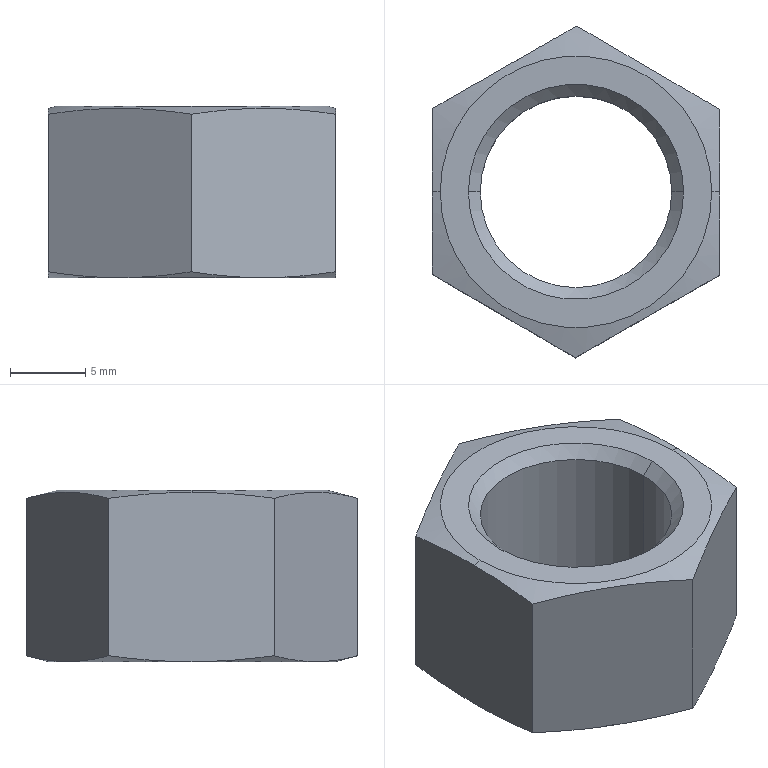Part | SolidWorks | features Cut 2, Chamfer 1, Extrusion 1 | 1 solid | 18 faces | box 19.096 x 22 x 11.38 mm | volume 2097 mm3 | cone 8 | plane 8 | cylinder 2 | commonest cylinder face diameters 12.7 x2
STEP:
#1=CARTESIAN_POINT('',(-6.35,0.,10.594));
#2=VERTEX_POINT('',#1);
#3=CARTESIAN_POINT('',(6.35,0.,10.594));
#4=VERTEX_POINT('',#3);
#5=CARTESIAN_POINT('',(0.,0.,10.594));
#6=DIRECTION('',(0.,0.,1.));
#7=DIRECTION('',(-1.,0.,0.));
#8=AXIS2_PLACEMENT_3D('',#5,#6,#7);
#9=CIRCLE('',#8,6.35);
#10=EDGE_CURVE('',#2,#4,#9,.T.);
#11=ORIENTED_EDGE('',*,*,#10,.F.);
#12=CARTESIAN_POINT('',(-7.136,0.,11.38));
#13=VERTEX_POINT('',#12);
#14=CARTESIAN_POINT('',(-6.35,0.,10.594));
#15=DIRECTION('',(-0.7071,0.,0.7071));
#16=VECTOR('',#15,1000.);
#17=LINE('',#14,#16);
#18=EDGE_CURVE('',#2,#13,#17,.T.);
#19=ORIENTED_EDGE('',*,*,#18,.T.);
#20=CARTESIAN_POINT('',(7.136,0.,11.38));
#21=VERTEX_POINT('',#20);
#22=CARTESIAN_POINT('',(0.,0.,11.38));
#23=DIRECTION('',(0.,0.,-1.));
#24=DIRECTION('',(-1.,0.,0.));
#25=AXIS2_PLACEMENT_3D('',#22,#23,#24);
#26=CIRCLE('',#25,7.136);
#27=EDGE_CURVE('',#21,#13,#26,.T.);
#28=ORIENTED_EDGE('',*,*,#27,.F.);
#29=CARTESIAN_POINT('',(6.35,0.,10.594));
#30=DIRECTION('',(0.7071,0.,0.7071));
#31=VECTOR('',#30,1000.);
#32=LINE('',#29,#31);
#33=EDGE_CURVE('',#4,#21,#32,.T.);
#34=ORIENTED_EDGE('',*,*,#33,.F.);
#35=EDGE_LOOP('',(#11,#19,#28,#34));
#36=FACE_OUTER_BOUND('',#35,.T.);
#37=CARTESIAN_POINT('',(0.,0.,10.594));
#38=DIRECTION('',(0.,0.,1.));
#39=DIRECTION('',(1.,0.,0.));
#40=AXIS2_PLACEMENT_3D('',#37,#38,#39);
#41=CONICAL_SURFACE('',#40,6.35,0.7854);
#42=ADVANCED_FACE('',(#36),#41,.F.);
#43=CARTESIAN_POINT('',(6.35,0.,0.7857));
#44=VERTEX_POINT('',#43);
#45=CARTESIAN_POINT('',(-6.35,0.,0.7857));
#46=VERTEX_POINT('',#45);
#47=CARTESIAN_POINT('',(0.,0.,0.7857));
#48=DIRECTION('',(0.,0.,-1.));
#49=DIRECTION('',(-1.,0.,0.));
#50=AXIS2_PLACEMENT_3D('',#47,#48,#49);
#51=CIRCLE('',#50,6.35);
#52=EDGE_CURVE('',#44,#46,#51,.T.);
#53=ORIENTED_EDGE('',*,*,#52,.F.);
#54=CARTESIAN_POINT('',(7.136,0.,0.));
#55=VERTEX_POINT('',#54);
#56=CARTESIAN_POINT('',(7.136,0.,0.));
#57=DIRECTION('',(0.7071,0.,-0.7071));
#58=VECTOR('',#57,1000.);
#59=LINE('',#56,#58);
#60=EDGE_CURVE('',#44,#55,#59,.T.);
#61=ORIENTED_EDGE('',*,*,#60,.T.);
#62=CARTESIAN_POINT('',(-7.136,0.,0.));
#63=VERTEX_POINT('',#62);
#64=CARTESIAN_POINT('',(0.,0.,0.));
#65=DIRECTION('',(0.,0.,1.));
#66=DIRECTION('',(-1.,0.,0.));
#67=AXIS2_PLACEMENT_3D('',#64,#65,#66);
#68=CIRCLE('',#67,7.136);
#69=EDGE_CURVE('',#63,#55,#68,.T.);
#70=ORIENTED_EDGE('',*,*,#69,.F.);
#71=CARTESIAN_POINT('',(-7.136,0.,0.));
#72=DIRECTION('',(-0.7071,0.,-0.7071));
#73=VECTOR('',#72,1000.);
#74=LINE('',#71,#73);
#75=EDGE_CURVE('',#46,#63,#74,.T.);
#76=ORIENTED_EDGE('',*,*,#75,.F.);
#77=EDGE_LOOP('',(#53,#61,#70,#76));
#78=FACE_OUTER_BOUND('',#77,.T.);
#79=CARTESIAN_POINT('',(0.,0.,0.));
#80=DIRECTION('',(0.,0.,-1.));
#81=DIRECTION('',(-1.,0.,0.));
#82=AXIS2_PLACEMENT_3D('',#79,#80,#81);
#83=CONICAL_SURFACE('',#82,7.136,0.7854);
#84=ADVANCED_FACE('',(#78),#83,.F.);
#85=CARTESIAN_POINT('',(-9.,0.,11.38));
#86=VERTEX_POINT('',#85);
#87=CARTESIAN_POINT('',(9.,0.,11.38));
#88=VERTEX_POINT('',#87);
#89=CARTESIAN_POINT('',(0.,0.,11.38));
#90=DIRECTION('',(0.,0.,1.));
#91=DIRECTION('',(1.,0.,0.));
#92=AXIS2_PLACEMENT_3D('',#89,#90,#91);
#93=CIRCLE('',#92,9.);
#94=EDGE_CURVE('',#86,#88,#93,.T.);
#95=ORIENTED_EDGE('',*,*,#94,.F.);
#96=CARTESIAN_POINT('',(-9.526,0.,11.239));
#97=VERTEX_POINT('',#96);
#98=CARTESIAN_POINT('',(-9.,0.,11.38));
#99=DIRECTION('',(-0.9659,0.,-0.2588));
#100=VECTOR('',#99,1000.);
#101=LINE('',#98,#100);
#102=EDGE_CURVE('',#86,#97,#101,.T.);
#103=ORIENTED_EDGE('',*,*,#102,.T.);
#104=CARTESIAN_POINT('',(-9.548,-5.462,10.844));
#105=VERTEX_POINT('',#104);
#106=CARTESIAN_POINT('',(-9.526,0.,11.239));
#107=CARTESIAN_POINT('',(-9.53,-0.9104,11.238));
#108=CARTESIAN_POINT('',(-9.534,-1.821,11.201));
#109=CARTESIAN_POINT('',(-9.541,-3.642,11.065));
#110=CARTESIAN_POINT('',(-9.544,-4.552,10.966));
#111=CARTESIAN_POINT('',(-9.548,-5.462,10.844));
#112=B_SPLINE_CURVE_WITH_KNOTS('',3,(#106,#107,#108,#109,#110,#111),.UNSPECIFIED.,.F.,.F.,(4,2,4),(0.005538,0.008269,0.011),.UNSPECIFIED.);
#113=EDGE_CURVE('',#97,#105,#112,.T.);
#114=ORIENTED_EDGE('',*,*,#113,.T.);
#115=CARTESIAN_POINT('',(-0.04327,-11.,10.844));
#116=VERTEX_POINT('',#115);
#117=CARTESIAN_POINT('',(-9.548,-5.462,10.844));
#118=CARTESIAN_POINT('',(-8.756,-5.924,10.967));
#119=CARTESIAN_POINT('',(-7.964,-6.385,11.067));
#120=CARTESIAN_POINT('',(-6.38,-7.308,11.203));
#121=CARTESIAN_POINT('',(-4.796,-8.231,11.275));
#122=CARTESIAN_POINT('',(-3.211,-9.154,11.203));
#123=CARTESIAN_POINT('',(-1.627,-10.077,11.067));
#124=CARTESIAN_POINT('',(-0.8353,-10.538,10.967));
#125=CARTESIAN_POINT('',(-0.04327,-11.,10.844));
#126=B_SPLINE_CURVE_WITH_KNOTS('',3,(#117,#118,#119,#120,#121,#122,#123,#124,#125),.UNSPECIFIED.,.F.,.F.,(4,2,1,2,4),(0.000000232,0.00275,0.0055,0.00825,0.011),.UNSPECIFIED.);
#127=EDGE_CURVE('',#105,#116,#126,.T.);
#128=ORIENTED_EDGE('',*,*,#127,.T.);
#129=CARTESIAN_POINT('',(9.505,-5.537,10.844));
#130=VERTEX_POINT('',#129);
#131=CARTESIAN_POINT('',(-0.04327,-11.,10.844));
#132=CARTESIAN_POINT('',(0.7524,-10.545,10.967));
#133=CARTESIAN_POINT('',(1.548,-10.09,11.067));
#134=CARTESIAN_POINT('',(3.139,-9.179,11.203));
#135=CARTESIAN_POINT('',(4.731,-8.269,11.275));
#136=CARTESIAN_POINT('',(6.322,-7.358,11.203));
#137=CARTESIAN_POINT('',(7.913,-6.448,11.067));
#138=CARTESIAN_POINT('',(8.709,-5.993,10.967));
#139=CARTESIAN_POINT('',(9.505,-5.537,10.844));
#140=B_SPLINE_CURVE_WITH_KNOTS('',3,(#131,#132,#133,#134,#135,#136,#137,#138,#139),.UNSPECIFIED.,.F.,.F.,(4,2,1,2,4),(0.00000023,0.00275,0.0055,0.00825,0.011),.UNSPECIFIED.);
#141=EDGE_CURVE('',#116,#130,#140,.T.);
#142=ORIENTED_EDGE('',*,*,#141,.T.);
#143=CARTESIAN_POINT('',(9.526,0.,11.239));
#144=VERTEX_POINT('',#143);
#145=CARTESIAN_POINT('',(9.505,-5.537,10.844));
#146=CARTESIAN_POINT('',(9.508,-4.615,10.968));
#147=CARTESIAN_POINT('',(9.512,-3.692,11.068));
#148=CARTESIAN_POINT('',(9.519,-1.846,11.204));
#149=CARTESIAN_POINT('',(9.523,-0.9229,11.24));
#150=CARTESIAN_POINT('',(9.526,0.,11.239));
#151=B_SPLINE_CURVE_WITH_KNOTS('',3,(#145,#146,#147,#148,#149,#150),.UNSPECIFIED.,.F.,.F.,(4,2,4),(0.0000002,0.002769,0.005538),.UNSPECIFIED.);
#152=EDGE_CURVE('',#130,#144,#151,.T.);
#153=ORIENTED_EDGE('',*,*,#152,.T.);
#154=CARTESIAN_POINT('',(9.,0.,11.38));
#155=DIRECTION('',(0.9659,0.,-0.2588));
#156=VECTOR('',#155,1000.);
#157=LINE('',#154,#156);
#158=EDGE_CURVE('',#88,#144,#157,.T.);
#159=ORIENTED_EDGE('',*,*,#158,.F.);
#160=EDGE_LOOP('',(#95,#103,#114,#128,#142,#153,#159));
#161=FACE_OUTER_BOUND('',#160,.T.);
#162=CARTESIAN_POINT('',(0.,0.,11.38));
#163=DIRECTION('',(0.,0.,-1.));
#164=DIRECTION('',(1.,0.,0.));
#165=AXIS2_PLACEMENT_3D('',#162,#163,#164);
#166=CONICAL_SURFACE('',#165,9.,1.309);
#167=ADVANCED_FACE('',(#161),#166,.T.);
#168=CARTESIAN_POINT('',(9.5,0.,0.));
#169=VERTEX_POINT('',#168);
#170=CARTESIAN_POINT('',(-9.5,0.,0.));
#171=VERTEX_POINT('',#170);
#172=CARTESIAN_POINT('',(0.,0.,0.));
#173=DIRECTION('',(0.,0.,-1.));
#174=DIRECTION('',(-1.,0.,0.));
#175=AXIS2_PLACEMENT_3D('',#172,#173,#174);
#176=CIRCLE('',#175,9.5);
#177=EDGE_CURVE('',#169,#171,#176,.T.);
#178=ORIENTED_EDGE('',*,*,#177,.F.);
#179=CARTESIAN_POINT('',(9.526,0.,0.007061));
#180=VERTEX_POINT('',#179);
#181=CARTESIAN_POINT('',(9.5,0.,0.));
#182=DIRECTION('',(0.9659,0.,0.2588));
#183=VECTOR('',#182,1000.);
#184=LINE('',#181,#183);
#185=EDGE_CURVE('',#169,#180,#184,.T.);
#186=ORIENTED_EDGE('',*,*,#185,.T.);
#187=CARTESIAN_POINT('',(9.505,-5.537,0.4019));
#188=VERTEX_POINT('',#187);
#189=CARTESIAN_POINT('',(9.526,0.,0.007061));
#190=CARTESIAN_POINT('',(9.523,-0.9229,0.006089));
#191=CARTESIAN_POINT('',(9.519,-1.846,0.04173));
#192=CARTESIAN_POINT('',(9.512,-3.692,0.178));
#193=CARTESIAN_POINT('',(9.508,-4.615,0.2783));
#194=CARTESIAN_POINT('',(9.505,-5.537,0.4019));
#195=B_SPLINE_CURVE_WITH_KNOTS('',3,(#189,#190,#191,#192,#193,#194),.UNSPECIFIED.,.F.,.F.,(4,2,4),(0.005463,0.008231,0.011),.UNSPECIFIED.);
#196=EDGE_CURVE('',#180,#188,#195,.T.);
#197=ORIENTED_EDGE('',*,*,#196,.T.);
#198=CARTESIAN_POINT('',(-0.04327,-11.,0.4019));
#199=VERTEX_POINT('',#198);
#200=CARTESIAN_POINT('',(9.505,-5.537,0.4019));
#201=CARTESIAN_POINT('',(8.709,-5.993,0.2791));
#202=CARTESIAN_POINT('',(7.913,-6.448,0.1794));
#203=CARTESIAN_POINT('',(6.322,-7.358,0.04315));
#204=CARTESIAN_POINT('',(4.731,-8.269,-0.02906));
#205=CARTESIAN_POINT('',(3.139,-9.179,0.04315));
#206=CARTESIAN_POINT('',(1.548,-10.09,0.1794));
#207=CARTESIAN_POINT('',(0.7524,-10.545,0.2791));
#208=CARTESIAN_POINT('',(-0.04327,-11.,0.4019));
#209=B_SPLINE_CURVE_WITH_KNOTS('',3,(#200,#201,#202,#203,#204,#205,#206,#207,#208),.UNSPECIFIED.,.F.,.F.,(4,2,1,2,4),(0.00000023,0.00275,0.0055,0.00825,0.011),.UNSPECIFIED.);
#210=EDGE_CURVE('',#188,#199,#209,.T.);
#211=ORIENTED_EDGE('',*,*,#210,.T.);
#212=CARTESIAN_POINT('',(-9.548,-5.462,0.4019));
#213=VERTEX_POINT('',#212);
#214=CARTESIAN_POINT('',(-0.04327,-11.,0.4019));
#215=CARTESIAN_POINT('',(-0.8353,-10.538,0.2791));
#216=CARTESIAN_POINT('',(-1.627,-10.077,0.1794));
#217=CARTESIAN_POINT('',(-3.211,-9.154,0.04315));
#218=CARTESIAN_POINT('',(-4.796,-8.231,-0.02906));
#219=CARTESIAN_POINT('',(-6.38,-7.308,0.04315));
#220=CARTESIAN_POINT('',(-7.964,-6.385,0.1794));
#221=CARTESIAN_POINT('',(-8.756,-5.924,0.2791));
#222=CARTESIAN_POINT('',(-9.548,-5.462,0.4019));
#223=B_SPLINE_CURVE_WITH_KNOTS('',3,(#214,#215,#216,#217,#218,#219,#220,#221,#222),.UNSPECIFIED.,.F.,.F.,(4,2,1,2,4),(0.000000232,0.00275,0.0055,0.00825,0.011),.UNSPECIFIED.);
#224=EDGE_CURVE('',#199,#213,#223,.T.);
#225=ORIENTED_EDGE('',*,*,#224,.T.);
#226=CARTESIAN_POINT('',(-9.526,0.,0.007061));
#227=VERTEX_POINT('',#226);
#228=CARTESIAN_POINT('',(-9.548,-5.462,0.4019));
#229=CARTESIAN_POINT('',(-9.544,-4.552,0.28));
#230=CARTESIAN_POINT('',(-9.541,-3.642,0.1808));
#231=CARTESIAN_POINT('',(-9.534,-1.821,0.04458));
#232=CARTESIAN_POINT('',(-9.53,-0.9104,0.008021));
#233=CARTESIAN_POINT('',(-9.526,0.,0.007061));
#234=B_SPLINE_CURVE_WITH_KNOTS('',3,(#228,#229,#230,#231,#232,#233),.UNSPECIFIED.,.F.,.F.,(4,2,4),(0.0000002,0.002731,0.005463),.UNSPECIFIED.);
#235=EDGE_CURVE('',#213,#227,#234,.T.);
#236=ORIENTED_EDGE('',*,*,#235,.T.);
#237=CARTESIAN_POINT('',(-9.5,0.,0.));
#238=DIRECTION('',(-0.9659,0.,0.2588));
#239=VECTOR('',#238,1000.);
#240=LINE('',#237,#239);
#241=EDGE_CURVE('',#171,#227,#240,.T.);
#242=ORIENTED_EDGE('',*,*,#241,.F.);
#243=EDGE_LOOP('',(#178,#186,#197,#211,#225,#236,#242));
#244=FACE_OUTER_BOUND('',#243,.T.);
#245=CARTESIAN_POINT('',(0.,0.,0.));
#246=DIRECTION('',(0.,0.,1.));
#247=DIRECTION('',(-1.,0.,0.));
#248=AXIS2_PLACEMENT_3D('',#245,#246,#247);
#249=CONICAL_SURFACE('',#248,9.5,1.309);
#250=ADVANCED_FACE('',(#244),#249,.T.);
#251=ORIENTED_EDGE('',*,*,#10,.T.);
#252=CARTESIAN_POINT('',(6.35,0.,11.38));
#253=DIRECTION('',(0.,0.,-1.));
#254=VECTOR('',#253,1000.);
#255=LINE('',#252,#254);
#256=EDGE_CURVE('',#4,#44,#255,.T.);
#257=ORIENTED_EDGE('',*,*,#256,.T.);
#258=ORIENTED_EDGE('',*,*,#52,.T.);
#259=CARTESIAN_POINT('',(-6.35,0.,11.38));
#260=DIRECTION('',(0.,0.,-1.));
#261=VECTOR('',#260,1000.);
#262=LINE('',#259,#261);
#263=EDGE_CURVE('',#2,#46,#262,.T.);
#264=ORIENTED_EDGE('',*,*,#263,.F.);
#265=EDGE_LOOP('',(#251,#257,#258,#264));
#266=FACE_OUTER_BOUND('',#265,.T.);
#267=CARTESIAN_POINT('',(0.,0.,11.38));
#268=DIRECTION('',(0.,0.,-1.));
#269=DIRECTION('',(-1.,0.,0.));
#270=AXIS2_PLACEMENT_3D('',#267,#268,#269);
#271=CYLINDRICAL_SURFACE('',#270,6.35);
#272=ADVANCED_FACE('',(#266),#271,.F.);
#273=CARTESIAN_POINT('',(9.548,5.462,10.844));
#274=VERTEX_POINT('',#273);
#275=CARTESIAN_POINT('',(0.04327,11.,10.844));
#276=VERTEX_POINT('',#275);
#277=CARTESIAN_POINT('',(9.548,5.462,10.844));
#278=CARTESIAN_POINT('',(8.756,5.924,10.967));
#279=CARTESIAN_POINT('',(7.964,6.385,11.067));
#280=CARTESIAN_POINT('',(6.38,7.308,11.203));
#281=CARTESIAN_POINT('',(4.796,8.231,11.275));
#282=CARTESIAN_POINT('',(3.211,9.154,11.203));
#283=CARTESIAN_POINT('',(1.627,10.077,11.067));
#284=CARTESIAN_POINT('',(0.8353,10.538,10.967));
#285=CARTESIAN_POINT('',(0.04327,11.,10.844));
#286=B_SPLINE_CURVE_WITH_KNOTS('',3,(#277,#278,#279,#280,#281,#282,#283,#284,#285),.UNSPECIFIED.,.F.,.F.,(4,2,1,2,4),(0.000000232,0.00275,0.0055,0.00825,0.011),.UNSPECIFIED.);
#287=EDGE_CURVE('',#274,#276,#286,.T.);
#288=ORIENTED_EDGE('',*,*,#287,.F.);
#289=CARTESIAN_POINT('',(9.548,5.462,0.4019));
#290=VERTEX_POINT('',#289);
#291=CARTESIAN_POINT('',(9.548,5.462,11.38));
#292=DIRECTION('',(0.,0.,-1.));
#293=VECTOR('',#292,1000.);
#294=LINE('',#291,#293);
#295=EDGE_CURVE('',#274,#290,#294,.T.);
#296=ORIENTED_EDGE('',*,*,#295,.T.);
#297=CARTESIAN_POINT('',(0.04327,11.,0.4019));
#298=VERTEX_POINT('',#297);
#299=CARTESIAN_POINT('',(0.04327,11.,0.4019));
#300=CARTESIAN_POINT('',(0.8353,10.538,0.2791));
#301=CARTESIAN_POINT('',(1.627,10.077,0.1794));
#302=CARTESIAN_POINT('',(3.211,9.154,0.04315));
#303=CARTESIAN_POINT('',(4.796,8.231,-0.02906));
#304=CARTESIAN_POINT('',(6.38,7.308,0.04315));
#305=CARTESIAN_POINT('',(7.964,6.385,0.1794));
#306=CARTESIAN_POINT('',(8.756,5.924,0.2791));
#307=CARTESIAN_POINT('',(9.548,5.462,0.4019));
#308=B_SPLINE_CURVE_WITH_KNOTS('',3,(#299,#300,#301,#302,#303,#304,#305,#306,#307),.UNSPECIFIED.,.F.,.F.,(4,2,1,2,4),(0.000000232,0.00275,0.0055,0.00825,0.011),.UNSPECIFIED.);
#309=EDGE_CURVE('',#298,#290,#308,.T.);
#310=ORIENTED_EDGE('',*,*,#309,.F.);
#311=CARTESIAN_POINT('',(0.04327,11.,11.38));
#312=DIRECTION('',(0.,0.,-1.));
#313=VECTOR('',#312,1000.);
#314=LINE('',#311,#313);
#315=EDGE_CURVE('',#276,#298,#314,.T.);
#316=ORIENTED_EDGE('',*,*,#315,.F.);
#317=EDGE_LOOP('',(#288,#296,#310,#316));
#318=FACE_OUTER_BOUND('',#317,.T.);
#319=CARTESIAN_POINT('',(9.548,5.462,11.38));
#320=DIRECTION('',(-0.5034,-0.8641,0.));
#321=DIRECTION('',(0.8641,-0.5034,0.));
#322=AXIS2_PLACEMENT_3D('',#319,#320,#321);
#323=PLANE('',#322);
#324=ADVANCED_FACE('',(#318),#323,.F.);
#325=CARTESIAN_POINT('',(-9.505,5.537,10.844));
#326=VERTEX_POINT('',#325);
#327=CARTESIAN_POINT('',(0.04327,11.,10.844));
#328=CARTESIAN_POINT('',(-0.7524,10.545,10.967));
#329=CARTESIAN_POINT('',(-1.548,10.09,11.067));
#330=CARTESIAN_POINT('',(-3.139,9.179,11.203));
#331=CARTESIAN_POINT('',(-4.731,8.269,11.275));
#332=CARTESIAN_POINT('',(-6.322,7.358,11.203));
#333=CARTESIAN_POINT('',(-7.913,6.448,11.067));
#334=CARTESIAN_POINT('',(-8.709,5.993,10.967));
#335=CARTESIAN_POINT('',(-9.505,5.537,10.844));
#336=B_SPLINE_CURVE_WITH_KNOTS('',3,(#327,#328,#329,#330,#331,#332,#333,#334,#335),.UNSPECIFIED.,.F.,.F.,(4,2,1,2,4),(0.00000023,0.00275,0.0055,0.00825,0.011),.UNSPECIFIED.);
#337=EDGE_CURVE('',#276,#326,#336,.T.);
#338=ORIENTED_EDGE('',*,*,#337,.F.);
#339=ORIENTED_EDGE('',*,*,#315,.T.);
#340=CARTESIAN_POINT('',(-9.505,5.537,0.4019));
#341=VERTEX_POINT('',#340);
#342=CARTESIAN_POINT('',(-9.505,5.537,0.4019));
#343=CARTESIAN_POINT('',(-8.709,5.993,0.2791));
#344=CARTESIAN_POINT('',(-7.913,6.448,0.1794));
#345=CARTESIAN_POINT('',(-6.322,7.358,0.04315));
#346=CARTESIAN_POINT('',(-4.731,8.269,-0.02906));
#347=CARTESIAN_POINT('',(-3.139,9.179,0.04315));
#348=CARTESIAN_POINT('',(-1.548,10.09,0.1794));
#349=CARTESIAN_POINT('',(-0.7524,10.545,0.2791));
#350=CARTESIAN_POINT('',(0.04327,11.,0.4019));
#351=B_SPLINE_CURVE_WITH_KNOTS('',3,(#342,#343,#344,#345,#346,#347,#348,#349,#350),.UNSPECIFIED.,.F.,.F.,(4,2,1,2,4),(0.00000023,0.00275,0.0055,0.00825,0.011),.UNSPECIFIED.);
#352=EDGE_CURVE('',#341,#298,#351,.T.);
#353=ORIENTED_EDGE('',*,*,#352,.F.);
#354=CARTESIAN_POINT('',(-9.505,5.537,11.38));
#355=DIRECTION('',(0.,0.,-1.));
#356=VECTOR('',#355,1000.);
#357=LINE('',#354,#356);
#358=EDGE_CURVE('',#326,#341,#357,.T.);
#359=ORIENTED_EDGE('',*,*,#358,.F.);
#360=EDGE_LOOP('',(#338,#339,#353,#359));
#361=FACE_OUTER_BOUND('',#360,.T.);
#362=CARTESIAN_POINT('',(0.04327,11.,11.38));
#363=DIRECTION('',(0.4966,-0.868,0.));
#364=DIRECTION('',(0.868,0.4966,0.));
#365=AXIS2_PLACEMENT_3D('',#362,#363,#364);
#366=PLANE('',#365);
#367=ADVANCED_FACE('',(#361),#366,.F.);
#368=CARTESIAN_POINT('',(-9.505,5.537,10.844));
#369=CARTESIAN_POINT('',(-9.508,4.615,10.968));
#370=CARTESIAN_POINT('',(-9.512,3.692,11.068));
#371=CARTESIAN_POINT('',(-9.519,1.846,11.204));
#372=CARTESIAN_POINT('',(-9.523,0.9229,11.24));
#373=CARTESIAN_POINT('',(-9.526,0.,11.239));
#374=B_SPLINE_CURVE_WITH_KNOTS('',3,(#368,#369,#370,#371,#372,#373),.UNSPECIFIED.,.F.,.F.,(4,2,4),(0.0000002,0.002769,0.005538),.UNSPECIFIED.);
#375=EDGE_CURVE('',#326,#97,#374,.T.);
#376=ORIENTED_EDGE('',*,*,#375,.F.);
#377=ORIENTED_EDGE('',*,*,#358,.T.);
#378=CARTESIAN_POINT('',(-9.526,0.,0.007061));
#379=CARTESIAN_POINT('',(-9.523,0.9229,0.006089));
#380=CARTESIAN_POINT('',(-9.519,1.846,0.04173));
#381=CARTESIAN_POINT('',(-9.512,3.692,0.178));
#382=CARTESIAN_POINT('',(-9.508,4.615,0.2783));
#383=CARTESIAN_POINT('',(-9.505,5.537,0.4019));
#384=B_SPLINE_CURVE_WITH_KNOTS('',3,(#378,#379,#380,#381,#382,#383),.UNSPECIFIED.,.F.,.F.,(4,2,4),(0.005463,0.008231,0.011),.UNSPECIFIED.);
#385=EDGE_CURVE('',#227,#341,#384,.T.);
#386=ORIENTED_EDGE('',*,*,#385,.F.);
#387=ORIENTED_EDGE('',*,*,#235,.F.);
#388=CARTESIAN_POINT('',(-9.548,-5.462,11.38));
#389=DIRECTION('',(0.,0.,-1.));
#390=VECTOR('',#389,1000.);
#391=LINE('',#388,#390);
#392=EDGE_CURVE('',#105,#213,#391,.T.);
#393=ORIENTED_EDGE('',*,*,#392,.F.);
#394=ORIENTED_EDGE('',*,*,#113,.F.);
#395=EDGE_LOOP('',(#376,#377,#386,#387,#393,#394));
#396=FACE_OUTER_BOUND('',#395,.T.);
#397=CARTESIAN_POINT('',(-9.505,5.537,11.38));
#398=DIRECTION('',(1.,-0.003934,0.));
#399=DIRECTION('',(0.003934,1.,0.));
#400=AXIS2_PLACEMENT_3D('',#397,#398,#399);
#401=PLANE('',#400);
#402=ADVANCED_FACE('',(#396),#401,.F.);
#403=ORIENTED_EDGE('',*,*,#127,.F.);
#404=ORIENTED_EDGE('',*,*,#392,.T.);
#405=ORIENTED_EDGE('',*,*,#224,.F.);
#406=CARTESIAN_POINT('',(-0.04327,-11.,11.38));
#407=DIRECTION('',(0.,0.,-1.));
#408=VECTOR('',#407,1000.);
#409=LINE('',#406,#408);
#410=EDGE_CURVE('',#116,#199,#409,.T.);
#411=ORIENTED_EDGE('',*,*,#410,.F.);
#412=EDGE_LOOP('',(#403,#404,#405,#411));
#413=FACE_OUTER_BOUND('',#412,.T.);
#414=CARTESIAN_POINT('',(-9.548,-5.462,11.38));
#415=DIRECTION('',(0.5034,0.8641,0.));
#416=DIRECTION('',(-0.8641,0.5034,0.));
#417=AXIS2_PLACEMENT_3D('',#414,#415,#416);
#418=PLANE('',#417);
#419=ADVANCED_FACE('',(#413),#418,.F.);
#420=ORIENTED_EDGE('',*,*,#141,.F.);
#421=ORIENTED_EDGE('',*,*,#410,.T.);
#422=ORIENTED_EDGE('',*,*,#210,.F.);
#423=CARTESIAN_POINT('',(9.505,-5.537,11.38));
#424=DIRECTION('',(0.,0.,-1.));
#425=VECTOR('',#424,1000.);
#426=LINE('',#423,#425);
#427=EDGE_CURVE('',#130,#188,#426,.T.);
#428=ORIENTED_EDGE('',*,*,#427,.F.);
#429=EDGE_LOOP('',(#420,#421,#422,#428));
#430=FACE_OUTER_BOUND('',#429,.T.);
#431=CARTESIAN_POINT('',(-0.04327,-11.,11.38));
#432=DIRECTION('',(-0.4966,0.868,0.));
#433=DIRECTION('',(-0.868,-0.4966,0.));
#434=AXIS2_PLACEMENT_3D('',#431,#432,#433);
#435=PLANE('',#434);
#436=ADVANCED_FACE('',(#430),#435,.F.);
#437=ORIENTED_EDGE('',*,*,#152,.F.);
#438=ORIENTED_EDGE('',*,*,#427,.T.);
#439=ORIENTED_EDGE('',*,*,#196,.F.);
#440=CARTESIAN_POINT('',(9.548,5.462,0.4019));
#441=CARTESIAN_POINT('',(9.544,4.552,0.28));
#442=CARTESIAN_POINT('',(9.541,3.642,0.1808));
#443=CARTESIAN_POINT('',(9.534,1.821,0.04458));
#444=CARTESIAN_POINT('',(9.53,0.9104,0.008021));
#445=CARTESIAN_POINT('',(9.526,0.,0.007061));
#446=B_SPLINE_CURVE_WITH_KNOTS('',3,(#440,#441,#442,#443,#444,#445),.UNSPECIFIED.,.F.,.F.,(4,2,4),(0.0000002,0.002731,0.005463),.UNSPECIFIED.);
#447=EDGE_CURVE('',#290,#180,#446,.T.);
#448=ORIENTED_EDGE('',*,*,#447,.F.);
#449=ORIENTED_EDGE('',*,*,#295,.F.);
#450=CARTESIAN_POINT('',(9.526,0.,11.239));
#451=CARTESIAN_POINT('',(9.53,0.9104,11.238));
#452=CARTESIAN_POINT('',(9.534,1.821,11.201));
#453=CARTESIAN_POINT('',(9.541,3.642,11.065));
#454=CARTESIAN_POINT('',(9.544,4.552,10.966));
#455=CARTESIAN_POINT('',(9.548,5.462,10.844));
#456=B_SPLINE_CURVE_WITH_KNOTS('',3,(#450,#451,#452,#453,#454,#455),.UNSPECIFIED.,.F.,.F.,(4,2,4),(0.005538,0.008269,0.011),.UNSPECIFIED.);
#457=EDGE_CURVE('',#144,#274,#456,.T.);
#458=ORIENTED_EDGE('',*,*,#457,.F.);
#459=EDGE_LOOP('',(#437,#438,#439,#448,#449,#458));
#460=FACE_OUTER_BOUND('',#459,.T.);
#461=CARTESIAN_POINT('',(9.505,-5.537,11.38));
#462=DIRECTION('',(-1.,0.003934,0.));
#463=DIRECTION('',(-0.003934,-1.,0.));
#464=AXIS2_PLACEMENT_3D('',#461,#462,#463);
#465=PLANE('',#464);
#466=ADVANCED_FACE('',(#460),#465,.F.);
#467=ORIENTED_EDGE('',*,*,#27,.T.);
#468=CARTESIAN_POINT('',(0.,0.,11.38));
#469=DIRECTION('',(0.,0.,-1.));
#470=DIRECTION('',(-1.,0.,0.));
#471=AXIS2_PLACEMENT_3D('',#468,#469,#470);
#472=CIRCLE('',#471,7.136);
#473=EDGE_CURVE('',#13,#21,#472,.T.);
#474=ORIENTED_EDGE('',*,*,#473,.T.);
#475=EDGE_LOOP('',(#467,#474));
#476=FACE_BOUND('',#475,.T.);
#477=CARTESIAN_POINT('',(0.,0.,11.38));
#478=DIRECTION('',(0.,0.,1.));
#479=DIRECTION('',(1.,0.,0.));
#480=AXIS2_PLACEMENT_3D('',#477,#478,#479);
#481=CIRCLE('',#480,9.);
#482=EDGE_CURVE('',#88,#86,#481,.T.);
#483=ORIENTED_EDGE('',*,*,#482,.T.);
#484=ORIENTED_EDGE('',*,*,#94,.T.);
#485=EDGE_LOOP('',(#483,#484));
#486=FACE_OUTER_BOUND('',#485,.T.);
#487=CARTESIAN_POINT('',(19.052,-0.07495,11.38));
#488=DIRECTION('',(0.,0.,-1.));
#489=DIRECTION('',(-1.,0.,0.));
#490=AXIS2_PLACEMENT_3D('',#487,#488,#489);
#491=PLANE('',#490);
#492=ADVANCED_FACE('',(#476,#486),#491,.F.);
#493=ORIENTED_EDGE('',*,*,#69,.T.);
#494=CARTESIAN_POINT('',(0.,0.,0.));
#495=DIRECTION('',(0.,0.,1.));
#496=DIRECTION('',(-1.,0.,0.));
#497=AXIS2_PLACEMENT_3D('',#494,#495,#496);
#498=CIRCLE('',#497,7.136);
#499=EDGE_CURVE('',#55,#63,#498,.T.);
#500=ORIENTED_EDGE('',*,*,#499,.T.);
#501=EDGE_LOOP('',(#493,#500));
#502=FACE_BOUND('',#501,.T.);
#503=CARTESIAN_POINT('',(0.,0.,0.));
#504=DIRECTION('',(0.,0.,-1.));
#505=DIRECTION('',(-1.,0.,0.));
#506=AXIS2_PLACEMENT_3D('',#503,#504,#505);
#507=CIRCLE('',#506,9.5);
#508=EDGE_CURVE('',#171,#169,#507,.T.);
#509=ORIENTED_EDGE('',*,*,#508,.T.);
#510=ORIENTED_EDGE('',*,*,#177,.T.);
#511=EDGE_LOOP('',(#509,#510));
#512=FACE_OUTER_BOUND('',#511,.T.);
#513=CARTESIAN_POINT('',(19.052,-0.07495,0.));
#514=DIRECTION('',(0.,0.,-1.));
#515=DIRECTION('',(-1.,0.,0.));
#516=AXIS2_PLACEMENT_3D('',#513,#514,#515);
#517=PLANE('',#516);
#518=ADVANCED_FACE('',(#502,#512),#517,.T.);
#519=ORIENTED_EDGE('',*,*,#256,.F.);
#520=CARTESIAN_POINT('',(0.,0.,10.594));
#521=DIRECTION('',(0.,0.,1.));
#522=DIRECTION('',(-1.,0.,0.));
#523=AXIS2_PLACEMENT_3D('',#520,#521,#522);
#524=CIRCLE('',#523,6.35);
#525=EDGE_CURVE('',#4,#2,#524,.T.);
#526=ORIENTED_EDGE('',*,*,#525,.T.);
#527=ORIENTED_EDGE('',*,*,#263,.T.);
#528=CARTESIAN_POINT('',(0.,0.,0.7857));
#529=DIRECTION('',(0.,0.,-1.));
#530=DIRECTION('',(-1.,0.,0.));
#531=AXIS2_PLACEMENT_3D('',#528,#529,#530);
#532=CIRCLE('',#531,6.35);
#533=EDGE_CURVE('',#46,#44,#532,.T.);
#534=ORIENTED_EDGE('',*,*,#533,.T.);
#535=EDGE_LOOP('',(#519,#526,#527,#534));
#536=FACE_OUTER_BOUND('',#535,.T.);
#537=CARTESIAN_POINT('',(0.,0.,11.38));
#538=DIRECTION('',(0.,0.,-1.));
#539=DIRECTION('',(-1.,0.,0.));
#540=AXIS2_PLACEMENT_3D('',#537,#538,#539);
#541=CYLINDRICAL_SURFACE('',#540,6.35);
#542=ADVANCED_FACE('',(#536),#541,.F.);
#543=ORIENTED_EDGE('',*,*,#185,.F.);
#544=ORIENTED_EDGE('',*,*,#508,.F.);
#545=ORIENTED_EDGE('',*,*,#241,.T.);
#546=ORIENTED_EDGE('',*,*,#385,.T.);
#547=ORIENTED_EDGE('',*,*,#352,.T.);
#548=ORIENTED_EDGE('',*,*,#309,.T.);
#549=ORIENTED_EDGE('',*,*,#447,.T.);
#550=EDGE_LOOP('',(#543,#544,#545,#546,#547,#548,#549));
#551=FACE_OUTER_BOUND('',#550,.T.);
#552=CARTESIAN_POINT('',(0.,0.,0.));
#553=DIRECTION('',(0.,0.,1.));
#554=DIRECTION('',(-1.,0.,0.));
#555=AXIS2_PLACEMENT_3D('',#552,#553,#554);
#556=CONICAL_SURFACE('',#555,9.5,1.309);
#557=ADVANCED_FACE('',(#551),#556,.T.);
#558=ORIENTED_EDGE('',*,*,#102,.F.);
#559=ORIENTED_EDGE('',*,*,#482,.F.);
#560=ORIENTED_EDGE('',*,*,#158,.T.);
#561=ORIENTED_EDGE('',*,*,#457,.T.);
#562=ORIENTED_EDGE('',*,*,#287,.T.);
#563=ORIENTED_EDGE('',*,*,#337,.T.);
#564=ORIENTED_EDGE('',*,*,#375,.T.);
#565=EDGE_LOOP('',(#558,#559,#560,#561,#562,#563,#564));
#566=FACE_OUTER_BOUND('',#565,.T.);
#567=CARTESIAN_POINT('',(0.,0.,11.38));
#568=DIRECTION('',(0.,0.,-1.));
#569=DIRECTION('',(1.,0.,0.));
#570=AXIS2_PLACEMENT_3D('',#567,#568,#569);
#571=CONICAL_SURFACE('',#570,9.,1.309);
#572=ADVANCED_FACE('',(#566),#571,.T.);
#573=ORIENTED_EDGE('',*,*,#60,.F.);
#574=ORIENTED_EDGE('',*,*,#533,.F.);
#575=ORIENTED_EDGE('',*,*,#75,.T.);
#576=ORIENTED_EDGE('',*,*,#499,.F.);
#577=EDGE_LOOP('',(#573,#574,#575,#576));
#578=FACE_OUTER_BOUND('',#577,.T.);
#579=CARTESIAN_POINT('',(0.,0.,0.));
#580=DIRECTION('',(0.,0.,-1.));
#581=DIRECTION('',(-1.,0.,0.));
#582=AXIS2_PLACEMENT_3D('',#579,#580,#581);
#583=CONICAL_SURFACE('',#582,7.136,0.7854);
#584=ADVANCED_FACE('',(#578),#583,.F.);
#585=ORIENTED_EDGE('',*,*,#18,.F.);
#586=ORIENTED_EDGE('',*,*,#525,.F.);
#587=ORIENTED_EDGE('',*,*,#33,.T.);
#588=ORIENTED_EDGE('',*,*,#473,.F.);
#589=EDGE_LOOP('',(#585,#586,#587,#588));
#590=FACE_OUTER_BOUND('',#589,.T.);
#591=CARTESIAN_POINT('',(0.,0.,10.594));
#592=DIRECTION('',(0.,0.,1.));
#593=DIRECTION('',(1.,0.,0.));
#594=AXIS2_PLACEMENT_3D('',#591,#592,#593);
#595=CONICAL_SURFACE('',#594,6.35,0.7854);
#596=ADVANCED_FACE('',(#590),#595,.F.);
#597=CLOSED_SHELL('',(#42,#84,#167,#250,#272,#324,#367,#402,#419,#436,#466,#492,#518,#542,#557,#572,#584,#596));
#598=MANIFOLD_SOLID_BREP('',#597);
#599=CARTESIAN_POINT('',(0.,0.,0.));
#600=DIRECTION('',(0.,0.,1.));
#601=DIRECTION('',(1.,0.,0.));
#602=AXIS2_PLACEMENT_3D('',#599,#600,#601);
#603=(LENGTH_UNIT()NAMED_UNIT(*)SI_UNIT(.MILLI.,.METRE.));
#604=UNCERTAINTY_MEASURE_WITH_UNIT(LENGTH_MEASURE(0.00001),#603,'','');
#605=(NAMED_UNIT(*)PLANE_ANGLE_UNIT()SI_UNIT($,.RADIAN.));
#606=(NAMED_UNIT(*)SI_UNIT($,.STERADIAN.)SOLID_ANGLE_UNIT());
#607=(GEOMETRIC_REPRESENTATION_CONTEXT(3)GLOBAL_UNCERTAINTY_ASSIGNED_CONTEXT((#604))GLOBAL_UNIT_ASSIGNED_CONTEXT((#603,#605,#606))REPRESENTATION_CONTEXT('',''));
#608=ADVANCED_BREP_SHAPE_REPRESENTATION('',(#598,#602),#607);